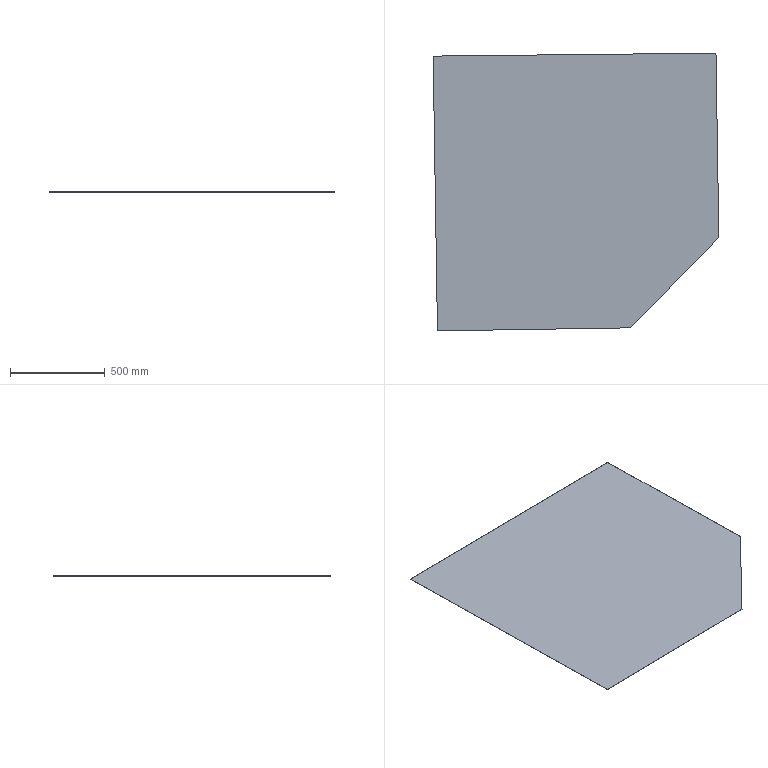Part | 1 solid | 7 faces | box 1505 x 1463 x 1.2 mm | volume 2449248 mm3 | plane 7
STEP:
#1=CARTESIAN_POINT('',(-275.3,-827.098,1404.5));
#2=VERTEX_POINT('',#1);
#3=CARTESIAN_POINT('',(743.934,-811.173,1404.5));
#4=VERTEX_POINT('',#3);
#5=CARTESIAN_POINT('',(743.934,-811.173,1404.5));
#6=DIRECTION('',(0.9999,0.01562,0.));
#7=VECTOR('',#6,1000.);
#8=LINE('',#5,#7);
#9=EDGE_CURVE('',#2,#4,#8,.T.);
#10=ORIENTED_EDGE('',*,*,#9,.T.);
#11=CARTESIAN_POINT('',(743.934,-811.173,1405.7));
#12=VERTEX_POINT('',#11);
#13=CARTESIAN_POINT('',(743.934,-811.173,1405.7));
#14=DIRECTION('',(0.,0.,-1.));
#15=VECTOR('',#14,1000.);
#16=LINE('',#13,#15);
#17=EDGE_CURVE('',#12,#4,#16,.T.);
#18=ORIENTED_EDGE('',*,*,#17,.F.);
#19=CARTESIAN_POINT('',(-275.3,-827.098,1405.7));
#20=VERTEX_POINT('',#19);
#21=CARTESIAN_POINT('',(743.934,-811.173,1405.7));
#22=DIRECTION('',(0.9999,0.01562,0.));
#23=VECTOR('',#22,1000.);
#24=LINE('',#21,#23);
#25=EDGE_CURVE('',#20,#12,#24,.T.);
#26=ORIENTED_EDGE('',*,*,#25,.F.);
#27=CARTESIAN_POINT('',(-275.3,-827.098,1405.7));
#28=DIRECTION('',(0.,0.,-1.));
#29=VECTOR('',#28,1000.);
#30=LINE('',#27,#29);
#31=EDGE_CURVE('',#20,#2,#30,.T.);
#32=ORIENTED_EDGE('',*,*,#31,.T.);
#33=EDGE_LOOP('',(#10,#18,#26,#32));
#34=FACE_OUTER_BOUND('',#33,.T.);
#35=CARTESIAN_POINT('',(743.934,-811.173,1405.7));
#36=DIRECTION('',(-0.01562,0.9999,0.));
#37=DIRECTION('',(0.,0.,1.));
#38=AXIS2_PLACEMENT_3D('',#35,#36,#37);
#39=PLANE('',#38);
#40=ADVANCED_FACE('',(#34),#39,.F.);
#41=CARTESIAN_POINT('',(1207.193,-335.011,1404.5));
#42=VERTEX_POINT('',#41);
#43=CARTESIAN_POINT('',(1207.193,-335.011,1404.5));
#44=DIRECTION('',(0.6973,0.7168,0.));
#45=VECTOR('',#44,1000.);
#46=LINE('',#43,#45);
#47=EDGE_CURVE('',#4,#42,#46,.T.);
#48=ORIENTED_EDGE('',*,*,#47,.T.);
#49=CARTESIAN_POINT('',(1207.193,-335.011,1405.7));
#50=VERTEX_POINT('',#49);
#51=CARTESIAN_POINT('',(1207.193,-335.011,1405.7));
#52=DIRECTION('',(0.,0.,-1.));
#53=VECTOR('',#52,1000.);
#54=LINE('',#51,#53);
#55=EDGE_CURVE('',#50,#42,#54,.T.);
#56=ORIENTED_EDGE('',*,*,#55,.F.);
#57=CARTESIAN_POINT('',(1207.193,-335.011,1405.7));
#58=DIRECTION('',(0.6973,0.7168,0.));
#59=VECTOR('',#58,1000.);
#60=LINE('',#57,#59);
#61=EDGE_CURVE('',#12,#50,#60,.T.);
#62=ORIENTED_EDGE('',*,*,#61,.F.);
#63=ORIENTED_EDGE('',*,*,#17,.T.);
#64=EDGE_LOOP('',(#48,#56,#62,#63));
#65=FACE_OUTER_BOUND('',#64,.T.);
#66=CARTESIAN_POINT('',(1207.193,-335.011,1405.7));
#67=DIRECTION('',(-0.7168,0.6973,0.));
#68=DIRECTION('',(0.,0.,1.));
#69=AXIS2_PLACEMENT_3D('',#66,#67,#68);
#70=PLANE('',#69);
#71=ADVANCED_FACE('',(#65),#70,.F.);
#72=CARTESIAN_POINT('',(1192.021,636.004,1404.5));
#73=VERTEX_POINT('',#72);
#74=CARTESIAN_POINT('',(1192.021,636.004,1404.5));
#75=DIRECTION('',(-0.01562,0.9999,0.));
#76=VECTOR('',#75,1000.);
#77=LINE('',#74,#76);
#78=EDGE_CURVE('',#42,#73,#77,.T.);
#79=ORIENTED_EDGE('',*,*,#78,.T.);
#80=CARTESIAN_POINT('',(1192.021,636.004,1405.7));
#81=VERTEX_POINT('',#80);
#82=CARTESIAN_POINT('',(1192.021,636.004,1405.7));
#83=DIRECTION('',(0.,0.,-1.));
#84=VECTOR('',#83,1000.);
#85=LINE('',#82,#84);
#86=EDGE_CURVE('',#81,#73,#85,.T.);
#87=ORIENTED_EDGE('',*,*,#86,.F.);
#88=CARTESIAN_POINT('',(1192.021,636.004,1405.7));
#89=DIRECTION('',(-0.01562,0.9999,0.));
#90=VECTOR('',#89,1000.);
#91=LINE('',#88,#90);
#92=EDGE_CURVE('',#50,#81,#91,.T.);
#93=ORIENTED_EDGE('',*,*,#92,.F.);
#94=ORIENTED_EDGE('',*,*,#55,.T.);
#95=EDGE_LOOP('',(#79,#87,#93,#94));
#96=FACE_OUTER_BOUND('',#95,.T.);
#97=CARTESIAN_POINT('',(1192.021,636.004,1405.7));
#98=DIRECTION('',(-0.9999,-0.01562,0.));
#99=DIRECTION('',(-0.01562,0.9999,0.));
#100=AXIS2_PLACEMENT_3D('',#97,#98,#99);
#101=PLANE('',#100);
#102=ADVANCED_FACE('',(#96),#101,.F.);
#103=CARTESIAN_POINT('',(-297.918,620.476,1404.5));
#104=VERTEX_POINT('',#103);
#105=CARTESIAN_POINT('',(-297.918,620.476,1404.5));
#106=DIRECTION('',(-0.9999,-0.01042,0.));
#107=VECTOR('',#106,1000.);
#108=LINE('',#105,#107);
#109=EDGE_CURVE('',#73,#104,#108,.T.);
#110=ORIENTED_EDGE('',*,*,#109,.T.);
#111=CARTESIAN_POINT('',(-297.918,620.476,1405.7));
#112=VERTEX_POINT('',#111);
#113=CARTESIAN_POINT('',(-297.918,620.476,1405.7));
#114=DIRECTION('',(0.,0.,-1.));
#115=VECTOR('',#114,1000.);
#116=LINE('',#113,#115);
#117=EDGE_CURVE('',#112,#104,#116,.T.);
#118=ORIENTED_EDGE('',*,*,#117,.F.);
#119=CARTESIAN_POINT('',(-297.918,620.476,1405.7));
#120=DIRECTION('',(-0.9999,-0.01042,0.));
#121=VECTOR('',#120,1000.);
#122=LINE('',#119,#121);
#123=EDGE_CURVE('',#81,#112,#122,.T.);
#124=ORIENTED_EDGE('',*,*,#123,.F.);
#125=ORIENTED_EDGE('',*,*,#86,.T.);
#126=EDGE_LOOP('',(#110,#118,#124,#125));
#127=FACE_OUTER_BOUND('',#126,.T.);
#128=CARTESIAN_POINT('',(-297.918,620.476,1405.7));
#129=DIRECTION('',(0.01042,-0.9999,0.));
#130=DIRECTION('',(0.,0.,-1.));
#131=AXIS2_PLACEMENT_3D('',#128,#129,#130);
#132=PLANE('',#131);
#133=ADVANCED_FACE('',(#127),#132,.F.);
#134=CARTESIAN_POINT('',(-275.3,-827.098,1404.5));
#135=DIRECTION('',(0.01562,-0.9999,0.));
#136=VECTOR('',#135,1000.);
#137=LINE('',#134,#136);
#138=EDGE_CURVE('',#104,#2,#137,.T.);
#139=ORIENTED_EDGE('',*,*,#138,.T.);
#140=ORIENTED_EDGE('',*,*,#31,.F.);
#141=CARTESIAN_POINT('',(-275.3,-827.098,1405.7));
#142=DIRECTION('',(0.01562,-0.9999,0.));
#143=VECTOR('',#142,1000.);
#144=LINE('',#141,#143);
#145=EDGE_CURVE('',#112,#20,#144,.T.);
#146=ORIENTED_EDGE('',*,*,#145,.F.);
#147=ORIENTED_EDGE('',*,*,#117,.T.);
#148=EDGE_LOOP('',(#139,#140,#146,#147));
#149=FACE_OUTER_BOUND('',#148,.T.);
#150=CARTESIAN_POINT('',(-275.3,-827.098,1405.7));
#151=DIRECTION('',(0.9999,0.01562,0.));
#152=DIRECTION('',(0.,0.,-1.));
#153=AXIS2_PLACEMENT_3D('',#150,#151,#152);
#154=PLANE('',#153);
#155=ADVANCED_FACE('',(#149),#154,.F.);
#156=ORIENTED_EDGE('',*,*,#25,.T.);
#157=ORIENTED_EDGE('',*,*,#61,.T.);
#158=ORIENTED_EDGE('',*,*,#92,.T.);
#159=ORIENTED_EDGE('',*,*,#123,.T.);
#160=ORIENTED_EDGE('',*,*,#145,.T.);
#161=EDGE_LOOP('',(#156,#157,#158,#159,#160));
#162=FACE_OUTER_BOUND('',#161,.T.);
#163=CARTESIAN_POINT('',(0.,0.,1405.7));
#164=DIRECTION('',(0.,0.,-1.));
#165=DIRECTION('',(0.,-1.,0.));
#166=AXIS2_PLACEMENT_3D('',#163,#164,#165);
#167=PLANE('',#166);
#168=ADVANCED_FACE('',(#162),#167,.F.);
#169=ORIENTED_EDGE('',*,*,#9,.F.);
#170=ORIENTED_EDGE('',*,*,#138,.F.);
#171=ORIENTED_EDGE('',*,*,#109,.F.);
#172=ORIENTED_EDGE('',*,*,#78,.F.);
#173=ORIENTED_EDGE('',*,*,#47,.F.);
#174=EDGE_LOOP('',(#169,#170,#171,#172,#173));
#175=FACE_OUTER_BOUND('',#174,.T.);
#176=CARTESIAN_POINT('',(0.,0.,1404.5));
#177=DIRECTION('',(0.,0.,-1.));
#178=DIRECTION('',(0.,-1.,0.));
#179=AXIS2_PLACEMENT_3D('',#176,#177,#178);
#180=PLANE('',#179);
#181=ADVANCED_FACE('',(#175),#180,.T.);
#182=CLOSED_SHELL('',(#40,#71,#102,#133,#155,#168,#181));
#183=MANIFOLD_SOLID_BREP('',#182);
#184=CARTESIAN_POINT('',(0.,0.,0.));
#185=DIRECTION('',(0.,0.,1.));
#186=DIRECTION('',(1.,0.,0.));
#187=AXIS2_PLACEMENT_3D('',#184,#185,#186);
#188=(LENGTH_UNIT()NAMED_UNIT(*)SI_UNIT(.MILLI.,.METRE.));
#189=UNCERTAINTY_MEASURE_WITH_UNIT(LENGTH_MEASURE(0.00001),#188,'','');
#190=(NAMED_UNIT(*)PLANE_ANGLE_UNIT()SI_UNIT($,.RADIAN.));
#191=(NAMED_UNIT(*)SI_UNIT($,.STERADIAN.)SOLID_ANGLE_UNIT());
#192=(GEOMETRIC_REPRESENTATION_CONTEXT(3)GLOBAL_UNCERTAINTY_ASSIGNED_CONTEXT((#189))GLOBAL_UNIT_ASSIGNED_CONTEXT((#188,#190,#191))REPRESENTATION_CONTEXT('',''));
#193=ADVANCED_BREP_SHAPE_REPRESENTATION('',(#183,#187),#192);